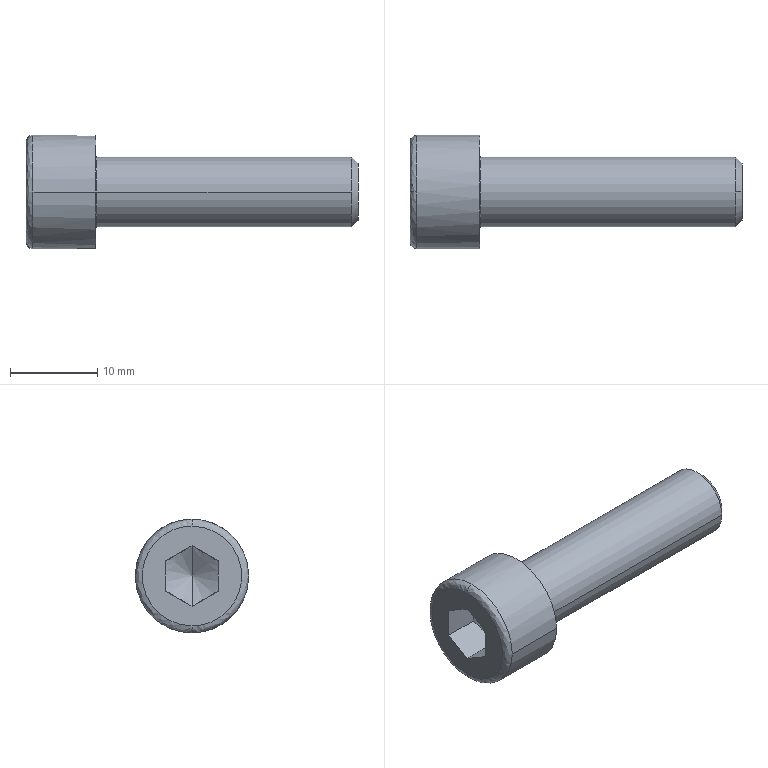Part | STEP file | AS 1420 - Metric M8 x 30 | 1 solid | 21 faces | box 38 x 13 x 13 mm | volume 2408 mm3 | plane 9 | spline 4 | cylinder 4 | cone 4 | commonest cylinder face diameters 8 x2 13 x2